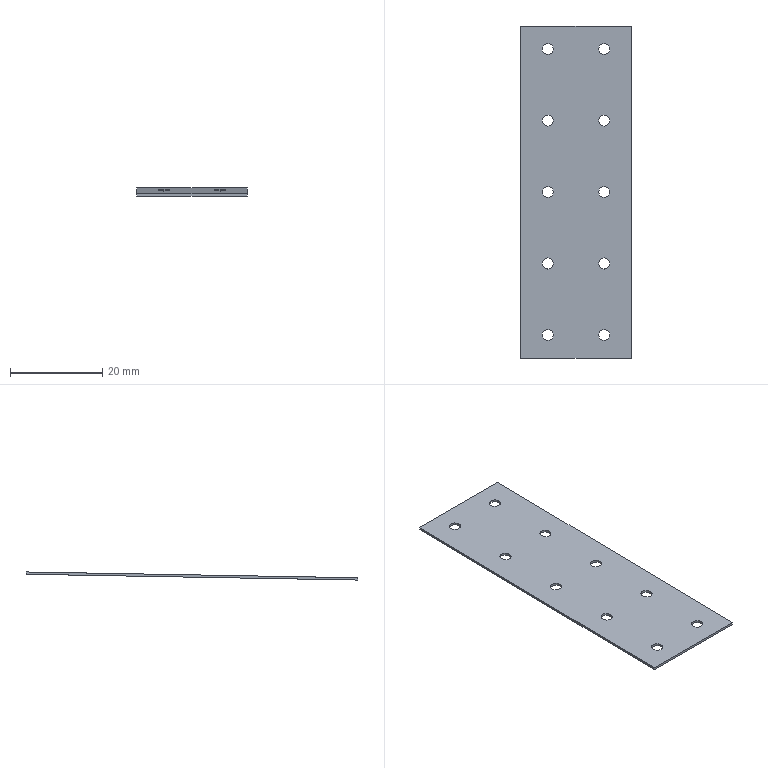Part | SolidWorks | features BaseBody 1 | 1 solid | 26 faces | box 24 x 71.993 x 1.756 mm | volume 841.326 mm3 | cylinder 20 | plane 6 | commonest cylinder face diameters 2.4 x20
STEP:
#1=CARTESIAN_POINT('',(-1405.625,-3.837,-0.5671));
#2=VERTEX_POINT('',#1);
#3=CARTESIAN_POINT('',(-1405.625,-1.437,-0.5252));
#4=VERTEX_POINT('',#3);
#5=CARTESIAN_POINT('',(-1405.625,-2.637,-0.5461));
#6=DIRECTION('',(0.,0.01745,-0.9998));
#7=DIRECTION('',(0.,-0.9998,-0.01745));
#8=AXIS2_PLACEMENT_3D('',#5,#6,#7);
#9=CIRCLE('',#8,1.2);
#10=EDGE_CURVE('',#2,#4,#9,.T.);
#11=ORIENTED_EDGE('',*,*,#10,.T.);
#12=CARTESIAN_POINT('',(-1405.625,-1.446,-0.02524));
#13=VERTEX_POINT('',#12);
#14=CARTESIAN_POINT('',(-1405.625,-1.437,-0.5252));
#15=DIRECTION('',(0.,-0.01745,0.9998));
#16=VECTOR('',#15,1000.);
#17=LINE('',#14,#16);
#18=EDGE_CURVE('',#4,#13,#17,.T.);
#19=ORIENTED_EDGE('',*,*,#18,.T.);
#20=CARTESIAN_POINT('',(-1405.625,-3.846,-0.06713));
#21=VERTEX_POINT('',#20);
#22=CARTESIAN_POINT('',(-1405.625,-2.646,-0.04619));
#23=DIRECTION('',(0.,-0.01745,0.9998));
#24=DIRECTION('',(0.,-0.9998,-0.01745));
#25=AXIS2_PLACEMENT_3D('',#22,#23,#24);
#26=CIRCLE('',#25,1.2);
#27=EDGE_CURVE('',#13,#21,#26,.T.);
#28=ORIENTED_EDGE('',*,*,#27,.T.);
#29=CARTESIAN_POINT('',(-1405.625,-3.837,-0.5671));
#30=DIRECTION('',(0.,-0.01745,0.9998));
#31=VECTOR('',#30,1000.);
#32=LINE('',#29,#31);
#33=EDGE_CURVE('',#2,#21,#32,.T.);
#34=ORIENTED_EDGE('',*,*,#33,.F.);
#35=EDGE_LOOP('',(#11,#19,#28,#34));
#36=FACE_OUTER_BOUND('',#35,.T.);
#37=CARTESIAN_POINT('',(-1405.625,-2.637,-0.5461));
#38=DIRECTION('',(0.,-0.01745,0.9998));
#39=DIRECTION('',(0.,-0.9998,-0.01745));
#40=AXIS2_PLACEMENT_3D('',#37,#38,#39);
#41=CYLINDRICAL_SURFACE('',#40,1.2);
#42=ADVANCED_FACE('',(#36),#41,.F.);
#43=CARTESIAN_POINT('',(-1417.875,27.156,-0.02607));
#44=VERTEX_POINT('',#43);
#45=CARTESIAN_POINT('',(-1417.875,29.556,0.01582));
#46=VERTEX_POINT('',#45);
#47=CARTESIAN_POINT('',(-1417.875,28.356,-0.005126));
#48=DIRECTION('',(0.,0.01745,-0.9998));
#49=DIRECTION('',(0.,-0.9998,-0.01745));
#50=AXIS2_PLACEMENT_3D('',#47,#48,#49);
#51=CIRCLE('',#50,1.2);
#52=EDGE_CURVE('',#44,#46,#51,.T.);
#53=ORIENTED_EDGE('',*,*,#52,.T.);
#54=CARTESIAN_POINT('',(-1417.875,29.547,0.5157));
#55=VERTEX_POINT('',#54);
#56=CARTESIAN_POINT('',(-1417.875,29.556,0.01582));
#57=DIRECTION('',(0.,-0.01745,0.9998));
#58=VECTOR('',#57,1000.);
#59=LINE('',#56,#58);
#60=EDGE_CURVE('',#46,#55,#59,.T.);
#61=ORIENTED_EDGE('',*,*,#60,.T.);
#62=CARTESIAN_POINT('',(-1417.875,27.147,0.4739));
#63=VERTEX_POINT('',#62);
#64=CARTESIAN_POINT('',(-1417.875,28.347,0.4948));
#65=DIRECTION('',(0.,0.01745,-0.9998));
#66=DIRECTION('',(0.,-0.9998,-0.01745));
#67=AXIS2_PLACEMENT_3D('',#64,#65,#66);
#68=CIRCLE('',#67,1.2);
#69=EDGE_CURVE('',#63,#55,#68,.T.);
#70=ORIENTED_EDGE('',*,*,#69,.F.);
#71=CARTESIAN_POINT('',(-1417.875,27.156,-0.02607));
#72=DIRECTION('',(0.,-0.01745,0.9998));
#73=VECTOR('',#72,1000.);
#74=LINE('',#71,#73);
#75=EDGE_CURVE('',#44,#63,#74,.T.);
#76=ORIENTED_EDGE('',*,*,#75,.F.);
#77=EDGE_LOOP('',(#53,#61,#70,#76));
#78=FACE_OUTER_BOUND('',#77,.T.);
#79=CARTESIAN_POINT('',(-1417.875,28.356,-0.005126));
#80=DIRECTION('',(0.,-0.01745,0.9998));
#81=DIRECTION('',(0.,-0.9998,-0.01745));
#82=AXIS2_PLACEMENT_3D('',#79,#80,#81);
#83=CYLINDRICAL_SURFACE('',#82,1.2);
#84=ADVANCED_FACE('',(#78),#83,.F.);
#85=CARTESIAN_POINT('',(-1417.875,11.659,-0.2966));
#86=VERTEX_POINT('',#85);
#87=CARTESIAN_POINT('',(-1417.875,14.059,-0.2547));
#88=VERTEX_POINT('',#87);
#89=CARTESIAN_POINT('',(-1417.875,12.859,-0.2756));
#90=DIRECTION('',(0.,0.01745,-0.9998));
#91=DIRECTION('',(0.,-0.9998,-0.01745));
#92=AXIS2_PLACEMENT_3D('',#89,#90,#91);
#93=CIRCLE('',#92,1.2);
#94=EDGE_CURVE('',#86,#88,#93,.T.);
#95=ORIENTED_EDGE('',*,*,#94,.T.);
#96=CARTESIAN_POINT('',(-1417.875,14.05,0.2452));
#97=VERTEX_POINT('',#96);
#98=CARTESIAN_POINT('',(-1417.875,14.059,-0.2547));
#99=DIRECTION('',(0.,-0.01745,0.9998));
#100=VECTOR('',#99,1000.);
#101=LINE('',#98,#100);
#102=EDGE_CURVE('',#88,#97,#101,.T.);
#103=ORIENTED_EDGE('',*,*,#102,.T.);
#104=CARTESIAN_POINT('',(-1417.875,11.651,0.2034));
#105=VERTEX_POINT('',#104);
#106=CARTESIAN_POINT('',(-1417.875,12.85,0.2243));
#107=DIRECTION('',(0.,0.01745,-0.9998));
#108=DIRECTION('',(0.,-0.9998,-0.01745));
#109=AXIS2_PLACEMENT_3D('',#106,#107,#108);
#110=CIRCLE('',#109,1.2);
#111=EDGE_CURVE('',#105,#97,#110,.T.);
#112=ORIENTED_EDGE('',*,*,#111,.F.);
#113=CARTESIAN_POINT('',(-1417.875,11.659,-0.2966));
#114=DIRECTION('',(0.,-0.01745,0.9998));
#115=VECTOR('',#114,1000.);
#116=LINE('',#113,#115);
#117=EDGE_CURVE('',#86,#105,#116,.T.);
#118=ORIENTED_EDGE('',*,*,#117,.F.);
#119=EDGE_LOOP('',(#95,#103,#112,#118));
#120=FACE_OUTER_BOUND('',#119,.T.);
#121=CARTESIAN_POINT('',(-1417.875,12.859,-0.2756));
#122=DIRECTION('',(0.,-0.01745,0.9998));
#123=DIRECTION('',(0.,-0.9998,-0.01745));
#124=AXIS2_PLACEMENT_3D('',#121,#122,#123);
#125=CYLINDRICAL_SURFACE('',#124,1.2);
#126=ADVANCED_FACE('',(#120),#125,.F.);
#127=CARTESIAN_POINT('',(-1405.625,-19.334,-0.8375));
#128=VERTEX_POINT('',#127);
#129=CARTESIAN_POINT('',(-1405.625,-16.934,-0.7957));
#130=VERTEX_POINT('',#129);
#131=CARTESIAN_POINT('',(-1405.625,-18.134,-0.8166));
#132=DIRECTION('',(0.,0.01745,-0.9998));
#133=DIRECTION('',(0.,-0.9998,-0.01745));
#134=AXIS2_PLACEMENT_3D('',#131,#132,#133);
#135=CIRCLE('',#134,1.2);
#136=EDGE_CURVE('',#128,#130,#135,.T.);
#137=ORIENTED_EDGE('',*,*,#136,.T.);
#138=CARTESIAN_POINT('',(-1405.625,-16.943,-0.2957));
#139=VERTEX_POINT('',#138);
#140=CARTESIAN_POINT('',(-1405.625,-16.934,-0.7957));
#141=DIRECTION('',(0.,-0.01745,0.9998));
#142=VECTOR('',#141,1000.);
#143=LINE('',#140,#142);
#144=EDGE_CURVE('',#130,#139,#143,.T.);
#145=ORIENTED_EDGE('',*,*,#144,.T.);
#146=CARTESIAN_POINT('',(-1405.625,-19.342,-0.3376));
#147=VERTEX_POINT('',#146);
#148=CARTESIAN_POINT('',(-1405.625,-18.143,-0.3167));
#149=DIRECTION('',(0.,0.01745,-0.9998));
#150=DIRECTION('',(0.,-0.9998,-0.01745));
#151=AXIS2_PLACEMENT_3D('',#148,#149,#150);
#152=CIRCLE('',#151,1.2);
#153=EDGE_CURVE('',#147,#139,#152,.T.);
#154=ORIENTED_EDGE('',*,*,#153,.F.);
#155=CARTESIAN_POINT('',(-1405.625,-19.334,-0.8375));
#156=DIRECTION('',(0.,-0.01745,0.9998));
#157=VECTOR('',#156,1000.);
#158=LINE('',#155,#157);
#159=EDGE_CURVE('',#128,#147,#158,.T.);
#160=ORIENTED_EDGE('',*,*,#159,.F.);
#161=EDGE_LOOP('',(#137,#145,#154,#160));
#162=FACE_OUTER_BOUND('',#161,.T.);
#163=CARTESIAN_POINT('',(-1405.625,-18.134,-0.8166));
#164=DIRECTION('',(0.,-0.01745,0.9998));
#165=DIRECTION('',(0.,-0.9998,-0.01745));
#166=AXIS2_PLACEMENT_3D('',#163,#164,#165);
#167=CYLINDRICAL_SURFACE('',#166,1.2);
#168=ADVANCED_FACE('',(#162),#167,.F.);
#169=CARTESIAN_POINT('',(-1417.875,42.652,0.2444));
#170=VERTEX_POINT('',#169);
#171=CARTESIAN_POINT('',(-1417.875,45.052,0.2863));
#172=VERTEX_POINT('',#171);
#173=CARTESIAN_POINT('',(-1417.875,43.852,0.2654));
#174=DIRECTION('',(0.,0.01745,-0.9998));
#175=DIRECTION('',(0.,-0.9998,-0.01745));
#176=AXIS2_PLACEMENT_3D('',#173,#174,#175);
#177=CIRCLE('',#176,1.2);
#178=EDGE_CURVE('',#170,#172,#177,.T.);
#179=ORIENTED_EDGE('',*,*,#178,.T.);
#180=CARTESIAN_POINT('',(-1417.875,45.043,0.7862));
#181=VERTEX_POINT('',#180);
#182=CARTESIAN_POINT('',(-1417.875,45.052,0.2863));
#183=DIRECTION('',(0.,-0.01745,0.9998));
#184=VECTOR('',#183,1000.);
#185=LINE('',#182,#184);
#186=EDGE_CURVE('',#172,#181,#185,.T.);
#187=ORIENTED_EDGE('',*,*,#186,.T.);
#188=CARTESIAN_POINT('',(-1417.875,42.644,0.7443));
#189=VERTEX_POINT('',#188);
#190=CARTESIAN_POINT('',(-1417.875,43.843,0.7653));
#191=DIRECTION('',(0.,0.01745,-0.9998));
#192=DIRECTION('',(0.,-0.9998,-0.01745));
#193=AXIS2_PLACEMENT_3D('',#190,#191,#192);
#194=CIRCLE('',#193,1.2);
#195=EDGE_CURVE('',#189,#181,#194,.T.);
#196=ORIENTED_EDGE('',*,*,#195,.F.);
#197=CARTESIAN_POINT('',(-1417.875,42.652,0.2444));
#198=DIRECTION('',(0.,-0.01745,0.9998));
#199=VECTOR('',#198,1000.);
#200=LINE('',#197,#199);
#201=EDGE_CURVE('',#170,#189,#200,.T.);
#202=ORIENTED_EDGE('',*,*,#201,.F.);
#203=EDGE_LOOP('',(#179,#187,#196,#202));
#204=FACE_OUTER_BOUND('',#203,.T.);
#205=CARTESIAN_POINT('',(-1417.875,43.852,0.2654));
#206=DIRECTION('',(0.,-0.01745,0.9998));
#207=DIRECTION('',(0.,-0.9998,-0.01745));
#208=AXIS2_PLACEMENT_3D('',#205,#206,#207);
#209=CYLINDRICAL_SURFACE('',#208,1.2);
#210=ADVANCED_FACE('',(#204),#209,.F.);
#211=CARTESIAN_POINT('',(-1405.625,42.652,0.2444));
#212=VERTEX_POINT('',#211);
#213=CARTESIAN_POINT('',(-1405.625,45.052,0.2863));
#214=VERTEX_POINT('',#213);
#215=CARTESIAN_POINT('',(-1405.625,43.852,0.2654));
#216=DIRECTION('',(0.,0.01745,-0.9998));
#217=DIRECTION('',(0.,-0.9998,-0.01745));
#218=AXIS2_PLACEMENT_3D('',#215,#216,#217);
#219=CIRCLE('',#218,1.2);
#220=EDGE_CURVE('',#212,#214,#219,.T.);
#221=ORIENTED_EDGE('',*,*,#220,.T.);
#222=CARTESIAN_POINT('',(-1405.625,45.043,0.7862));
#223=VERTEX_POINT('',#222);
#224=CARTESIAN_POINT('',(-1405.625,45.052,0.2863));
#225=DIRECTION('',(0.,-0.01745,0.9998));
#226=VECTOR('',#225,1000.);
#227=LINE('',#224,#226);
#228=EDGE_CURVE('',#214,#223,#227,.T.);
#229=ORIENTED_EDGE('',*,*,#228,.T.);
#230=CARTESIAN_POINT('',(-1405.625,42.644,0.7443));
#231=VERTEX_POINT('',#230);
#232=CARTESIAN_POINT('',(-1405.625,43.843,0.7653));
#233=DIRECTION('',(0.,0.01745,-0.9998));
#234=DIRECTION('',(0.,-0.9998,-0.01745));
#235=AXIS2_PLACEMENT_3D('',#232,#233,#234);
#236=CIRCLE('',#235,1.2);
#237=EDGE_CURVE('',#231,#223,#236,.T.);
#238=ORIENTED_EDGE('',*,*,#237,.F.);
#239=CARTESIAN_POINT('',(-1405.625,42.652,0.2444));
#240=DIRECTION('',(0.,-0.01745,0.9998));
#241=VECTOR('',#240,1000.);
#242=LINE('',#239,#241);
#243=EDGE_CURVE('',#212,#231,#242,.T.);
#244=ORIENTED_EDGE('',*,*,#243,.F.);
#245=EDGE_LOOP('',(#221,#229,#238,#244));
#246=FACE_OUTER_BOUND('',#245,.T.);
#247=CARTESIAN_POINT('',(-1405.625,43.852,0.2654));
#248=DIRECTION('',(0.,-0.01745,0.9998));
#249=DIRECTION('',(0.,-0.9998,-0.01745));
#250=AXIS2_PLACEMENT_3D('',#247,#248,#249);
#251=CYLINDRICAL_SURFACE('',#250,1.2);
#252=ADVANCED_FACE('',(#246),#251,.F.);
#253=CARTESIAN_POINT('',(-1417.875,-19.334,-0.8375));
#254=VERTEX_POINT('',#253);
#255=CARTESIAN_POINT('',(-1417.875,-16.934,-0.7957));
#256=VERTEX_POINT('',#255);
#257=CARTESIAN_POINT('',(-1417.875,-18.134,-0.8166));
#258=DIRECTION('',(0.,0.01745,-0.9998));
#259=DIRECTION('',(0.,-0.9998,-0.01745));
#260=AXIS2_PLACEMENT_3D('',#257,#258,#259);
#261=CIRCLE('',#260,1.2);
#262=EDGE_CURVE('',#254,#256,#261,.T.);
#263=ORIENTED_EDGE('',*,*,#262,.T.);
#264=CARTESIAN_POINT('',(-1417.875,-16.943,-0.2957));
#265=VERTEX_POINT('',#264);
#266=CARTESIAN_POINT('',(-1417.875,-16.934,-0.7957));
#267=DIRECTION('',(0.,-0.01745,0.9998));
#268=VECTOR('',#267,1000.);
#269=LINE('',#266,#268);
#270=EDGE_CURVE('',#256,#265,#269,.T.);
#271=ORIENTED_EDGE('',*,*,#270,.T.);
#272=CARTESIAN_POINT('',(-1417.875,-19.342,-0.3376));
#273=VERTEX_POINT('',#272);
#274=CARTESIAN_POINT('',(-1417.875,-18.143,-0.3167));
#275=DIRECTION('',(0.,0.01745,-0.9998));
#276=DIRECTION('',(0.,-0.9998,-0.01745));
#277=AXIS2_PLACEMENT_3D('',#274,#275,#276);
#278=CIRCLE('',#277,1.2);
#279=EDGE_CURVE('',#273,#265,#278,.T.);
#280=ORIENTED_EDGE('',*,*,#279,.F.);
#281=CARTESIAN_POINT('',(-1417.875,-19.334,-0.8375));
#282=DIRECTION('',(0.,-0.01745,0.9998));
#283=VECTOR('',#282,1000.);
#284=LINE('',#281,#283);
#285=EDGE_CURVE('',#254,#273,#284,.T.);
#286=ORIENTED_EDGE('',*,*,#285,.F.);
#287=EDGE_LOOP('',(#263,#271,#280,#286));
#288=FACE_OUTER_BOUND('',#287,.T.);
#289=CARTESIAN_POINT('',(-1417.875,-18.134,-0.8166));
#290=DIRECTION('',(0.,-0.01745,0.9998));
#291=DIRECTION('',(0.,-0.9998,-0.01745));
#292=AXIS2_PLACEMENT_3D('',#289,#290,#291);
#293=CYLINDRICAL_SURFACE('',#292,1.2);
#294=ADVANCED_FACE('',(#288),#293,.F.);
#295=CARTESIAN_POINT('',(-1405.625,11.659,-0.2966));
#296=VERTEX_POINT('',#295);
#297=CARTESIAN_POINT('',(-1405.625,14.059,-0.2547));
#298=VERTEX_POINT('',#297);
#299=CARTESIAN_POINT('',(-1405.625,12.859,-0.2756));
#300=DIRECTION('',(0.,0.01745,-0.9998));
#301=DIRECTION('',(0.,-0.9998,-0.01745));
#302=AXIS2_PLACEMENT_3D('',#299,#300,#301);
#303=CIRCLE('',#302,1.2);
#304=EDGE_CURVE('',#296,#298,#303,.T.);
#305=ORIENTED_EDGE('',*,*,#304,.T.);
#306=CARTESIAN_POINT('',(-1405.625,14.05,0.2452));
#307=VERTEX_POINT('',#306);
#308=CARTESIAN_POINT('',(-1405.625,14.059,-0.2547));
#309=DIRECTION('',(0.,-0.01745,0.9998));
#310=VECTOR('',#309,1000.);
#311=LINE('',#308,#310);
#312=EDGE_CURVE('',#298,#307,#311,.T.);
#313=ORIENTED_EDGE('',*,*,#312,.T.);
#314=CARTESIAN_POINT('',(-1405.625,11.651,0.2034));
#315=VERTEX_POINT('',#314);
#316=CARTESIAN_POINT('',(-1405.625,12.85,0.2243));
#317=DIRECTION('',(0.,0.01745,-0.9998));
#318=DIRECTION('',(0.,-0.9998,-0.01745));
#319=AXIS2_PLACEMENT_3D('',#316,#317,#318);
#320=CIRCLE('',#319,1.2);
#321=EDGE_CURVE('',#315,#307,#320,.T.);
#322=ORIENTED_EDGE('',*,*,#321,.F.);
#323=CARTESIAN_POINT('',(-1405.625,11.659,-0.2966));
#324=DIRECTION('',(0.,-0.01745,0.9998));
#325=VECTOR('',#324,1000.);
#326=LINE('',#323,#325);
#327=EDGE_CURVE('',#296,#315,#326,.T.);
#328=ORIENTED_EDGE('',*,*,#327,.F.);
#329=EDGE_LOOP('',(#305,#313,#322,#328));
#330=FACE_OUTER_BOUND('',#329,.T.);
#331=CARTESIAN_POINT('',(-1405.625,12.859,-0.2756));
#332=DIRECTION('',(0.,-0.01745,0.9998));
#333=DIRECTION('',(0.,-0.9998,-0.01745));
#334=AXIS2_PLACEMENT_3D('',#331,#332,#333);
#335=CYLINDRICAL_SURFACE('',#334,1.2);
#336=ADVANCED_FACE('',(#330),#335,.F.);
#337=CARTESIAN_POINT('',(-1405.625,27.156,-0.02607));
#338=VERTEX_POINT('',#337);
#339=CARTESIAN_POINT('',(-1405.625,29.556,0.01582));
#340=VERTEX_POINT('',#339);
#341=CARTESIAN_POINT('',(-1405.625,28.356,-0.005126));
#342=DIRECTION('',(0.,0.01745,-0.9998));
#343=DIRECTION('',(0.,-0.9998,-0.01745));
#344=AXIS2_PLACEMENT_3D('',#341,#342,#343);
#345=CIRCLE('',#344,1.2);
#346=EDGE_CURVE('',#338,#340,#345,.T.);
#347=ORIENTED_EDGE('',*,*,#346,.T.);
#348=CARTESIAN_POINT('',(-1405.625,29.547,0.5157));
#349=VERTEX_POINT('',#348);
#350=CARTESIAN_POINT('',(-1405.625,29.556,0.01582));
#351=DIRECTION('',(0.,-0.01745,0.9998));
#352=VECTOR('',#351,1000.);
#353=LINE('',#350,#352);
#354=EDGE_CURVE('',#340,#349,#353,.T.);
#355=ORIENTED_EDGE('',*,*,#354,.T.);
#356=CARTESIAN_POINT('',(-1405.625,27.147,0.4739));
#357=VERTEX_POINT('',#356);
#358=CARTESIAN_POINT('',(-1405.625,28.347,0.4948));
#359=DIRECTION('',(0.,0.01745,-0.9998));
#360=DIRECTION('',(0.,-0.9998,-0.01745));
#361=AXIS2_PLACEMENT_3D('',#358,#359,#360);
#362=CIRCLE('',#361,1.2);
#363=EDGE_CURVE('',#357,#349,#362,.T.);
#364=ORIENTED_EDGE('',*,*,#363,.F.);
#365=CARTESIAN_POINT('',(-1405.625,27.156,-0.02607));
#366=DIRECTION('',(0.,-0.01745,0.9998));
#367=VECTOR('',#366,1000.);
#368=LINE('',#365,#367);
#369=EDGE_CURVE('',#338,#357,#368,.T.);
#370=ORIENTED_EDGE('',*,*,#369,.F.);
#371=EDGE_LOOP('',(#347,#355,#364,#370));
#372=FACE_OUTER_BOUND('',#371,.T.);
#373=CARTESIAN_POINT('',(-1405.625,28.356,-0.005126));
#374=DIRECTION('',(0.,-0.01745,0.9998));
#375=DIRECTION('',(0.,-0.9998,-0.01745));
#376=AXIS2_PLACEMENT_3D('',#373,#374,#375);
#377=CYLINDRICAL_SURFACE('',#376,1.2);
#378=ADVANCED_FACE('',(#372),#377,.F.);
#379=CARTESIAN_POINT('',(-1417.875,-3.837,-0.5671));
#380=VERTEX_POINT('',#379);
#381=CARTESIAN_POINT('',(-1417.875,-1.437,-0.5252));
#382=VERTEX_POINT('',#381);
#383=CARTESIAN_POINT('',(-1417.875,-2.637,-0.5461));
#384=DIRECTION('',(0.,0.01745,-0.9998));
#385=DIRECTION('',(0.,-0.9998,-0.01745));
#386=AXIS2_PLACEMENT_3D('',#383,#384,#385);
#387=CIRCLE('',#386,1.2);
#388=EDGE_CURVE('',#380,#382,#387,.T.);
#389=ORIENTED_EDGE('',*,*,#388,.T.);
#390=CARTESIAN_POINT('',(-1417.875,-1.446,-0.02524));
#391=VERTEX_POINT('',#390);
#392=CARTESIAN_POINT('',(-1417.875,-1.437,-0.5252));
#393=DIRECTION('',(0.,-0.01745,0.9998));
#394=VECTOR('',#393,1000.);
#395=LINE('',#392,#394);
#396=EDGE_CURVE('',#382,#391,#395,.T.);
#397=ORIENTED_EDGE('',*,*,#396,.T.);
#398=CARTESIAN_POINT('',(-1417.875,-3.846,-0.06713));
#399=VERTEX_POINT('',#398);
#400=CARTESIAN_POINT('',(-1417.875,-2.646,-0.04619));
#401=DIRECTION('',(0.,0.01745,-0.9998));
#402=DIRECTION('',(0.,-0.9998,-0.01745));
#403=AXIS2_PLACEMENT_3D('',#400,#401,#402);
#404=CIRCLE('',#403,1.2);
#405=EDGE_CURVE('',#399,#391,#404,.T.);
#406=ORIENTED_EDGE('',*,*,#405,.F.);
#407=CARTESIAN_POINT('',(-1417.875,-3.837,-0.5671));
#408=DIRECTION('',(0.,-0.01745,0.9998));
#409=VECTOR('',#408,1000.);
#410=LINE('',#407,#409);
#411=EDGE_CURVE('',#380,#399,#410,.T.);
#412=ORIENTED_EDGE('',*,*,#411,.F.);
#413=EDGE_LOOP('',(#389,#397,#406,#412));
#414=FACE_OUTER_BOUND('',#413,.T.);
#415=CARTESIAN_POINT('',(-1417.875,-2.637,-0.5461));
#416=DIRECTION('',(0.,-0.01745,0.9998));
#417=DIRECTION('',(0.,-0.9998,-0.01745));
#418=AXIS2_PLACEMENT_3D('',#415,#416,#417);
#419=CYLINDRICAL_SURFACE('',#418,1.2);
#420=ADVANCED_FACE('',(#414),#419,.F.);
#421=ORIENTED_EDGE('',*,*,#18,.F.);
#422=CARTESIAN_POINT('',(-1405.625,-2.637,-0.5461));
#423=DIRECTION('',(0.,0.01745,-0.9998));
#424=DIRECTION('',(0.,-0.9998,-0.01745));
#425=AXIS2_PLACEMENT_3D('',#422,#423,#424);
#426=CIRCLE('',#425,1.2);
#427=EDGE_CURVE('',#4,#2,#426,.T.);
#428=ORIENTED_EDGE('',*,*,#427,.T.);
#429=ORIENTED_EDGE('',*,*,#33,.T.);
#430=CARTESIAN_POINT('',(-1405.625,-2.646,-0.04619));
#431=DIRECTION('',(0.,-0.01745,0.9998));
#432=DIRECTION('',(0.,-0.9998,-0.01745));
#433=AXIS2_PLACEMENT_3D('',#430,#431,#432);
#434=CIRCLE('',#433,1.2);
#435=EDGE_CURVE('',#21,#13,#434,.T.);
#436=ORIENTED_EDGE('',*,*,#435,.T.);
#437=EDGE_LOOP('',(#421,#428,#429,#436));
#438=FACE_OUTER_BOUND('',#437,.T.);
#439=CARTESIAN_POINT('',(-1405.625,-2.637,-0.5461));
#440=DIRECTION('',(0.,-0.01745,0.9998));
#441=DIRECTION('',(0.,-0.9998,-0.01745));
#442=AXIS2_PLACEMENT_3D('',#439,#440,#441);
#443=CYLINDRICAL_SURFACE('',#442,1.2);
#444=ADVANCED_FACE('',(#438),#443,.F.);
#445=ORIENTED_EDGE('',*,*,#435,.F.);
#446=ORIENTED_EDGE('',*,*,#27,.F.);
#447=EDGE_LOOP('',(#445,#446));
#448=FACE_BOUND('',#447,.T.);
#449=ORIENTED_EDGE('',*,*,#69,.T.);
#450=CARTESIAN_POINT('',(-1417.875,28.347,0.4948));
#451=DIRECTION('',(0.,0.01745,-0.9998));
#452=DIRECTION('',(0.,-0.9998,-0.01745));
#453=AXIS2_PLACEMENT_3D('',#450,#451,#452);
#454=CIRCLE('',#453,1.2);
#455=EDGE_CURVE('',#55,#63,#454,.T.);
#456=ORIENTED_EDGE('',*,*,#455,.T.);
#457=EDGE_LOOP('',(#449,#456));
#458=FACE_BOUND('',#457,.T.);
#459=ORIENTED_EDGE('',*,*,#111,.T.);
#460=CARTESIAN_POINT('',(-1417.875,12.85,0.2243));
#461=DIRECTION('',(0.,0.01745,-0.9998));
#462=DIRECTION('',(0.,-0.9998,-0.01745));
#463=AXIS2_PLACEMENT_3D('',#460,#461,#462);
#464=CIRCLE('',#463,1.2);
#465=EDGE_CURVE('',#97,#105,#464,.T.);
#466=ORIENTED_EDGE('',*,*,#465,.T.);
#467=EDGE_LOOP('',(#459,#466));
#468=FACE_BOUND('',#467,.T.);
#469=ORIENTED_EDGE('',*,*,#153,.T.);
#470=CARTESIAN_POINT('',(-1405.625,-18.143,-0.3167));
#471=DIRECTION('',(0.,0.01745,-0.9998));
#472=DIRECTION('',(0.,-0.9998,-0.01745));
#473=AXIS2_PLACEMENT_3D('',#470,#471,#472);
#474=CIRCLE('',#473,1.2);
#475=EDGE_CURVE('',#139,#147,#474,.T.);
#476=ORIENTED_EDGE('',*,*,#475,.T.);
#477=EDGE_LOOP('',(#469,#476));
#478=FACE_BOUND('',#477,.T.);
#479=ORIENTED_EDGE('',*,*,#195,.T.);
#480=CARTESIAN_POINT('',(-1417.875,43.843,0.7653));
#481=DIRECTION('',(0.,0.01745,-0.9998));
#482=DIRECTION('',(0.,-0.9998,-0.01745));
#483=AXIS2_PLACEMENT_3D('',#480,#481,#482);
#484=CIRCLE('',#483,1.2);
#485=EDGE_CURVE('',#181,#189,#484,.T.);
#486=ORIENTED_EDGE('',*,*,#485,.T.);
#487=EDGE_LOOP('',(#479,#486));
#488=FACE_BOUND('',#487,.T.);
#489=ORIENTED_EDGE('',*,*,#237,.T.);
#490=CARTESIAN_POINT('',(-1405.625,43.843,0.7653));
#491=DIRECTION('',(0.,0.01745,-0.9998));
#492=DIRECTION('',(0.,-0.9998,-0.01745));
#493=AXIS2_PLACEMENT_3D('',#490,#491,#492);
#494=CIRCLE('',#493,1.2);
#495=EDGE_CURVE('',#223,#231,#494,.T.);
#496=ORIENTED_EDGE('',*,*,#495,.T.);
#497=EDGE_LOOP('',(#489,#496));
#498=FACE_BOUND('',#497,.T.);
#499=ORIENTED_EDGE('',*,*,#279,.T.);
#500=CARTESIAN_POINT('',(-1417.875,-18.143,-0.3167));
#501=DIRECTION('',(0.,0.01745,-0.9998));
#502=DIRECTION('',(0.,-0.9998,-0.01745));
#503=AXIS2_PLACEMENT_3D('',#500,#501,#502);
#504=CIRCLE('',#503,1.2);
#505=EDGE_CURVE('',#265,#273,#504,.T.);
#506=ORIENTED_EDGE('',*,*,#505,.T.);
#507=EDGE_LOOP('',(#499,#506));
#508=FACE_BOUND('',#507,.T.);
#509=ORIENTED_EDGE('',*,*,#321,.T.);
#510=CARTESIAN_POINT('',(-1405.625,12.85,0.2243));
#511=DIRECTION('',(0.,0.01745,-0.9998));
#512=DIRECTION('',(0.,-0.9998,-0.01745));
#513=AXIS2_PLACEMENT_3D('',#510,#511,#512);
#514=CIRCLE('',#513,1.2);
#515=EDGE_CURVE('',#307,#315,#514,.T.);
#516=ORIENTED_EDGE('',*,*,#515,.T.);
#517=EDGE_LOOP('',(#509,#516));
#518=FACE_BOUND('',#517,.T.);
#519=ORIENTED_EDGE('',*,*,#363,.T.);
#520=CARTESIAN_POINT('',(-1405.625,28.347,0.4948));
#521=DIRECTION('',(0.,0.01745,-0.9998));
#522=DIRECTION('',(0.,-0.9998,-0.01745));
#523=AXIS2_PLACEMENT_3D('',#520,#521,#522);
#524=CIRCLE('',#523,1.2);
#525=EDGE_CURVE('',#349,#357,#524,.T.);
#526=ORIENTED_EDGE('',*,*,#525,.T.);
#527=EDGE_LOOP('',(#519,#526));
#528=FACE_BOUND('',#527,.T.);
#529=ORIENTED_EDGE('',*,*,#405,.T.);
#530=CARTESIAN_POINT('',(-1417.875,-2.646,-0.04619));
#531=DIRECTION('',(0.,0.01745,-0.9998));
#532=DIRECTION('',(0.,-0.9998,-0.01745));
#533=AXIS2_PLACEMENT_3D('',#530,#531,#532);
#534=CIRCLE('',#533,1.2);
#535=EDGE_CURVE('',#391,#399,#534,.T.);
#536=ORIENTED_EDGE('',*,*,#535,.T.);
#537=EDGE_LOOP('',(#529,#536));
#538=FACE_BOUND('',#537,.T.);
#539=CARTESIAN_POINT('',(-1423.75,48.843,0.8526));
#540=VERTEX_POINT('',#539);
#541=CARTESIAN_POINT('',(-1423.75,-23.142,-0.4039));
#542=VERTEX_POINT('',#541);
#543=CARTESIAN_POINT('',(-1423.75,12.85,0.2243));
#544=DIRECTION('',(0.,-0.9998,-0.01745));
#545=VECTOR('',#544,1000.);
#546=LINE('',#543,#545);
#547=EDGE_CURVE('',#540,#542,#546,.T.);
#548=ORIENTED_EDGE('',*,*,#547,.T.);
#549=CARTESIAN_POINT('',(-1399.75,-23.142,-0.4039));
#550=VERTEX_POINT('',#549);
#551=CARTESIAN_POINT('',(-1411.75,-23.142,-0.4039));
#552=DIRECTION('',(1.,0.,0.));
#553=VECTOR('',#552,1000.);
#554=LINE('',#551,#553);
#555=EDGE_CURVE('',#542,#550,#554,.T.);
#556=ORIENTED_EDGE('',*,*,#555,.T.);
#557=CARTESIAN_POINT('',(-1399.75,48.843,0.8526));
#558=VERTEX_POINT('',#557);
#559=CARTESIAN_POINT('',(-1399.75,12.85,0.2243));
#560=DIRECTION('',(0.,0.9998,0.01745));
#561=VECTOR('',#560,1000.);
#562=LINE('',#559,#561);
#563=EDGE_CURVE('',#550,#558,#562,.T.);
#564=ORIENTED_EDGE('',*,*,#563,.T.);
#565=CARTESIAN_POINT('',(-1411.75,48.843,0.8526));
#566=DIRECTION('',(-1.,0.,0.));
#567=VECTOR('',#566,1000.);
#568=LINE('',#565,#567);
#569=EDGE_CURVE('',#558,#540,#568,.T.);
#570=ORIENTED_EDGE('',*,*,#569,.T.);
#571=EDGE_LOOP('',(#548,#556,#564,#570));
#572=FACE_OUTER_BOUND('',#571,.T.);
#573=CARTESIAN_POINT('',(-1423.75,48.843,0.8526));
#574=DIRECTION('',(0.,-0.01745,0.9998));
#575=DIRECTION('',(0.,-0.9998,-0.01745));
#576=AXIS2_PLACEMENT_3D('',#573,#574,#575);
#577=PLANE('',#576);
#578=ADVANCED_FACE('',(#448,#458,#468,#478,#488,#498,#508,#518,#528,#538,#572),#577,.T.);
#579=ORIENTED_EDGE('',*,*,#10,.F.);
#580=ORIENTED_EDGE('',*,*,#427,.F.);
#581=EDGE_LOOP('',(#579,#580));
#582=FACE_BOUND('',#581,.T.);
#583=ORIENTED_EDGE('',*,*,#52,.F.);
#584=CARTESIAN_POINT('',(-1417.875,28.356,-0.005126));
#585=DIRECTION('',(0.,0.01745,-0.9998));
#586=DIRECTION('',(0.,-0.9998,-0.01745));
#587=AXIS2_PLACEMENT_3D('',#584,#585,#586);
#588=CIRCLE('',#587,1.2);
#589=EDGE_CURVE('',#46,#44,#588,.T.);
#590=ORIENTED_EDGE('',*,*,#589,.F.);
#591=EDGE_LOOP('',(#583,#590));
#592=FACE_BOUND('',#591,.T.);
#593=ORIENTED_EDGE('',*,*,#94,.F.);
#594=CARTESIAN_POINT('',(-1417.875,12.859,-0.2756));
#595=DIRECTION('',(0.,0.01745,-0.9998));
#596=DIRECTION('',(0.,-0.9998,-0.01745));
#597=AXIS2_PLACEMENT_3D('',#594,#595,#596);
#598=CIRCLE('',#597,1.2);
#599=EDGE_CURVE('',#88,#86,#598,.T.);
#600=ORIENTED_EDGE('',*,*,#599,.F.);
#601=EDGE_LOOP('',(#593,#600));
#602=FACE_BOUND('',#601,.T.);
#603=ORIENTED_EDGE('',*,*,#136,.F.);
#604=CARTESIAN_POINT('',(-1405.625,-18.134,-0.8166));
#605=DIRECTION('',(0.,0.01745,-0.9998));
#606=DIRECTION('',(0.,-0.9998,-0.01745));
#607=AXIS2_PLACEMENT_3D('',#604,#605,#606);
#608=CIRCLE('',#607,1.2);
#609=EDGE_CURVE('',#130,#128,#608,.T.);
#610=ORIENTED_EDGE('',*,*,#609,.F.);
#611=EDGE_LOOP('',(#603,#610));
#612=FACE_BOUND('',#611,.T.);
#613=ORIENTED_EDGE('',*,*,#178,.F.);
#614=CARTESIAN_POINT('',(-1417.875,43.852,0.2654));
#615=DIRECTION('',(0.,0.01745,-0.9998));
#616=DIRECTION('',(0.,-0.9998,-0.01745));
#617=AXIS2_PLACEMENT_3D('',#614,#615,#616);
#618=CIRCLE('',#617,1.2);
#619=EDGE_CURVE('',#172,#170,#618,.T.);
#620=ORIENTED_EDGE('',*,*,#619,.F.);
#621=EDGE_LOOP('',(#613,#620));
#622=FACE_BOUND('',#621,.T.);
#623=ORIENTED_EDGE('',*,*,#220,.F.);
#624=CARTESIAN_POINT('',(-1405.625,43.852,0.2654));
#625=DIRECTION('',(0.,0.01745,-0.9998));
#626=DIRECTION('',(0.,-0.9998,-0.01745));
#627=AXIS2_PLACEMENT_3D('',#624,#625,#626);
#628=CIRCLE('',#627,1.2);
#629=EDGE_CURVE('',#214,#212,#628,.T.);
#630=ORIENTED_EDGE('',*,*,#629,.F.);
#631=EDGE_LOOP('',(#623,#630));
#632=FACE_BOUND('',#631,.T.);
#633=ORIENTED_EDGE('',*,*,#262,.F.);
#634=CARTESIAN_POINT('',(-1417.875,-18.134,-0.8166));
#635=DIRECTION('',(0.,0.01745,-0.9998));
#636=DIRECTION('',(0.,-0.9998,-0.01745));
#637=AXIS2_PLACEMENT_3D('',#634,#635,#636);
#638=CIRCLE('',#637,1.2);
#639=EDGE_CURVE('',#256,#254,#638,.T.);
#640=ORIENTED_EDGE('',*,*,#639,.F.);
#641=EDGE_LOOP('',(#633,#640));
#642=FACE_BOUND('',#641,.T.);
#643=ORIENTED_EDGE('',*,*,#304,.F.);
#644=CARTESIAN_POINT('',(-1405.625,12.859,-0.2756));
#645=DIRECTION('',(0.,0.01745,-0.9998));
#646=DIRECTION('',(0.,-0.9998,-0.01745));
#647=AXIS2_PLACEMENT_3D('',#644,#645,#646);
#648=CIRCLE('',#647,1.2);
#649=EDGE_CURVE('',#298,#296,#648,.T.);
#650=ORIENTED_EDGE('',*,*,#649,.F.);
#651=EDGE_LOOP('',(#643,#650));
#652=FACE_BOUND('',#651,.T.);
#653=ORIENTED_EDGE('',*,*,#346,.F.);
#654=CARTESIAN_POINT('',(-1405.625,28.356,-0.005126));
#655=DIRECTION('',(0.,0.01745,-0.9998));
#656=DIRECTION('',(0.,-0.9998,-0.01745));
#657=AXIS2_PLACEMENT_3D('',#654,#655,#656);
#658=CIRCLE('',#657,1.2);
#659=EDGE_CURVE('',#340,#338,#658,.T.);
#660=ORIENTED_EDGE('',*,*,#659,.F.);
#661=EDGE_LOOP('',(#653,#660));
#662=FACE_BOUND('',#661,.T.);
#663=ORIENTED_EDGE('',*,*,#388,.F.);
#664=CARTESIAN_POINT('',(-1417.875,-2.637,-0.5461));
#665=DIRECTION('',(0.,0.01745,-0.9998));
#666=DIRECTION('',(0.,-0.9998,-0.01745));
#667=AXIS2_PLACEMENT_3D('',#664,#665,#666);
#668=CIRCLE('',#667,1.2);
#669=EDGE_CURVE('',#382,#380,#668,.T.);
#670=ORIENTED_EDGE('',*,*,#669,.F.);
#671=EDGE_LOOP('',(#663,#670));
#672=FACE_BOUND('',#671,.T.);
#673=CARTESIAN_POINT('',(-1423.75,-23.133,-0.9039));
#674=VERTEX_POINT('',#673);
#675=CARTESIAN_POINT('',(-1399.75,-23.133,-0.9039));
#676=VERTEX_POINT('',#675);
#677=CARTESIAN_POINT('',(-1411.75,-23.133,-0.9039));
#678=DIRECTION('',(1.,0.,0.));
#679=VECTOR('',#678,1000.);
#680=LINE('',#677,#679);
#681=EDGE_CURVE('',#674,#676,#680,.T.);
#682=ORIENTED_EDGE('',*,*,#681,.F.);
#683=CARTESIAN_POINT('',(-1423.75,48.851,0.3526));
#684=VERTEX_POINT('',#683);
#685=CARTESIAN_POINT('',(-1423.75,12.859,-0.2756));
#686=DIRECTION('',(0.,-0.9998,-0.01745));
#687=VECTOR('',#686,1000.);
#688=LINE('',#685,#687);
#689=EDGE_CURVE('',#684,#674,#688,.T.);
#690=ORIENTED_EDGE('',*,*,#689,.F.);
#691=CARTESIAN_POINT('',(-1399.75,48.851,0.3526));
#692=VERTEX_POINT('',#691);
#693=CARTESIAN_POINT('',(-1411.75,48.851,0.3526));
#694=DIRECTION('',(-1.,0.,0.));
#695=VECTOR('',#694,1000.);
#696=LINE('',#693,#695);
#697=EDGE_CURVE('',#692,#684,#696,.T.);
#698=ORIENTED_EDGE('',*,*,#697,.F.);
#699=CARTESIAN_POINT('',(-1399.75,12.859,-0.2756));
#700=DIRECTION('',(0.,0.9998,0.01745));
#701=VECTOR('',#700,1000.);
#702=LINE('',#699,#701);
#703=EDGE_CURVE('',#676,#692,#702,.T.);
#704=ORIENTED_EDGE('',*,*,#703,.F.);
#705=EDGE_LOOP('',(#682,#690,#698,#704));
#706=FACE_OUTER_BOUND('',#705,.T.);
#707=CARTESIAN_POINT('',(-1423.75,48.851,0.3526));
#708=DIRECTION('',(0.,-0.01745,0.9998));
#709=DIRECTION('',(0.,-0.9998,-0.01745));
#710=AXIS2_PLACEMENT_3D('',#707,#708,#709);
#711=PLANE('',#710);
#712=ADVANCED_FACE('',(#582,#592,#602,#612,#622,#632,#642,#652,#662,#672,#706),#711,.F.);
#713=ORIENTED_EDGE('',*,*,#60,.F.);
#714=ORIENTED_EDGE('',*,*,#589,.T.);
#715=ORIENTED_EDGE('',*,*,#75,.T.);
#716=ORIENTED_EDGE('',*,*,#455,.F.);
#717=EDGE_LOOP('',(#713,#714,#715,#716));
#718=FACE_OUTER_BOUND('',#717,.T.);
#719=CARTESIAN_POINT('',(-1417.875,28.356,-0.005126));
#720=DIRECTION('',(0.,-0.01745,0.9998));
#721=DIRECTION('',(0.,-0.9998,-0.01745));
#722=AXIS2_PLACEMENT_3D('',#719,#720,#721);
#723=CYLINDRICAL_SURFACE('',#722,1.2);
#724=ADVANCED_FACE('',(#718),#723,.F.);
#725=ORIENTED_EDGE('',*,*,#102,.F.);
#726=ORIENTED_EDGE('',*,*,#599,.T.);
#727=ORIENTED_EDGE('',*,*,#117,.T.);
#728=ORIENTED_EDGE('',*,*,#465,.F.);
#729=EDGE_LOOP('',(#725,#726,#727,#728));
#730=FACE_OUTER_BOUND('',#729,.T.);
#731=CARTESIAN_POINT('',(-1417.875,12.859,-0.2756));
#732=DIRECTION('',(0.,-0.01745,0.9998));
#733=DIRECTION('',(0.,-0.9998,-0.01745));
#734=AXIS2_PLACEMENT_3D('',#731,#732,#733);
#735=CYLINDRICAL_SURFACE('',#734,1.2);
#736=ADVANCED_FACE('',(#730),#735,.F.);
#737=ORIENTED_EDGE('',*,*,#144,.F.);
#738=ORIENTED_EDGE('',*,*,#609,.T.);
#739=ORIENTED_EDGE('',*,*,#159,.T.);
#740=ORIENTED_EDGE('',*,*,#475,.F.);
#741=EDGE_LOOP('',(#737,#738,#739,#740));
#742=FACE_OUTER_BOUND('',#741,.T.);
#743=CARTESIAN_POINT('',(-1405.625,-18.134,-0.8166));
#744=DIRECTION('',(0.,-0.01745,0.9998));
#745=DIRECTION('',(0.,-0.9998,-0.01745));
#746=AXIS2_PLACEMENT_3D('',#743,#744,#745);
#747=CYLINDRICAL_SURFACE('',#746,1.2);
#748=ADVANCED_FACE('',(#742),#747,.F.);
#749=ORIENTED_EDGE('',*,*,#186,.F.);
#750=ORIENTED_EDGE('',*,*,#619,.T.);
#751=ORIENTED_EDGE('',*,*,#201,.T.);
#752=ORIENTED_EDGE('',*,*,#485,.F.);
#753=EDGE_LOOP('',(#749,#750,#751,#752));
#754=FACE_OUTER_BOUND('',#753,.T.);
#755=CARTESIAN_POINT('',(-1417.875,43.852,0.2654));
#756=DIRECTION('',(0.,-0.01745,0.9998));
#757=DIRECTION('',(0.,-0.9998,-0.01745));
#758=AXIS2_PLACEMENT_3D('',#755,#756,#757);
#759=CYLINDRICAL_SURFACE('',#758,1.2);
#760=ADVANCED_FACE('',(#754),#759,.F.);
#761=ORIENTED_EDGE('',*,*,#228,.F.);
#762=ORIENTED_EDGE('',*,*,#629,.T.);
#763=ORIENTED_EDGE('',*,*,#243,.T.);
#764=ORIENTED_EDGE('',*,*,#495,.F.);
#765=EDGE_LOOP('',(#761,#762,#763,#764));
#766=FACE_OUTER_BOUND('',#765,.T.);
#767=CARTESIAN_POINT('',(-1405.625,43.852,0.2654));
#768=DIRECTION('',(0.,-0.01745,0.9998));
#769=DIRECTION('',(0.,-0.9998,-0.01745));
#770=AXIS2_PLACEMENT_3D('',#767,#768,#769);
#771=CYLINDRICAL_SURFACE('',#770,1.2);
#772=ADVANCED_FACE('',(#766),#771,.F.);
#773=ORIENTED_EDGE('',*,*,#270,.F.);
#774=ORIENTED_EDGE('',*,*,#639,.T.);
#775=ORIENTED_EDGE('',*,*,#285,.T.);
#776=ORIENTED_EDGE('',*,*,#505,.F.);
#777=EDGE_LOOP('',(#773,#774,#775,#776));
#778=FACE_OUTER_BOUND('',#777,.T.);
#779=CARTESIAN_POINT('',(-1417.875,-18.134,-0.8166));
#780=DIRECTION('',(0.,-0.01745,0.9998));
#781=DIRECTION('',(0.,-0.9998,-0.01745));
#782=AXIS2_PLACEMENT_3D('',#779,#780,#781);
#783=CYLINDRICAL_SURFACE('',#782,1.2);
#784=ADVANCED_FACE('',(#778),#783,.F.);
#785=ORIENTED_EDGE('',*,*,#312,.F.);
#786=ORIENTED_EDGE('',*,*,#649,.T.);
#787=ORIENTED_EDGE('',*,*,#327,.T.);
#788=ORIENTED_EDGE('',*,*,#515,.F.);
#789=EDGE_LOOP('',(#785,#786,#787,#788));
#790=FACE_OUTER_BOUND('',#789,.T.);
#791=CARTESIAN_POINT('',(-1405.625,12.859,-0.2756));
#792=DIRECTION('',(0.,-0.01745,0.9998));
#793=DIRECTION('',(0.,-0.9998,-0.01745));
#794=AXIS2_PLACEMENT_3D('',#791,#792,#793);
#795=CYLINDRICAL_SURFACE('',#794,1.2);
#796=ADVANCED_FACE('',(#790),#795,.F.);
#797=ORIENTED_EDGE('',*,*,#354,.F.);
#798=ORIENTED_EDGE('',*,*,#659,.T.);
#799=ORIENTED_EDGE('',*,*,#369,.T.);
#800=ORIENTED_EDGE('',*,*,#525,.F.);
#801=EDGE_LOOP('',(#797,#798,#799,#800));
#802=FACE_OUTER_BOUND('',#801,.T.);
#803=CARTESIAN_POINT('',(-1405.625,28.356,-0.005126));
#804=DIRECTION('',(0.,-0.01745,0.9998));
#805=DIRECTION('',(0.,-0.9998,-0.01745));
#806=AXIS2_PLACEMENT_3D('',#803,#804,#805);
#807=CYLINDRICAL_SURFACE('',#806,1.2);
#808=ADVANCED_FACE('',(#802),#807,.F.);
#809=ORIENTED_EDGE('',*,*,#396,.F.);
#810=ORIENTED_EDGE('',*,*,#669,.T.);
#811=ORIENTED_EDGE('',*,*,#411,.T.);
#812=ORIENTED_EDGE('',*,*,#535,.F.);
#813=EDGE_LOOP('',(#809,#810,#811,#812));
#814=FACE_OUTER_BOUND('',#813,.T.);
#815=CARTESIAN_POINT('',(-1417.875,-2.637,-0.5461));
#816=DIRECTION('',(0.,-0.01745,0.9998));
#817=DIRECTION('',(0.,-0.9998,-0.01745));
#818=AXIS2_PLACEMENT_3D('',#815,#816,#817);
#819=CYLINDRICAL_SURFACE('',#818,1.2);
#820=ADVANCED_FACE('',(#814),#819,.F.);
#821=CARTESIAN_POINT('',(-1423.75,-23.137,-0.6539));
#822=DIRECTION('',(0.,-0.01745,0.9998));
#823=VECTOR('',#822,1000.);
#824=LINE('',#821,#823);
#825=EDGE_CURVE('',#674,#542,#824,.T.);
#826=ORIENTED_EDGE('',*,*,#825,.F.);
#827=ORIENTED_EDGE('',*,*,#681,.T.);
#828=CARTESIAN_POINT('',(-1399.75,-23.137,-0.6539));
#829=DIRECTION('',(0.,0.01745,-0.9998));
#830=VECTOR('',#829,1000.);
#831=LINE('',#828,#830);
#832=EDGE_CURVE('',#550,#676,#831,.T.);
#833=ORIENTED_EDGE('',*,*,#832,.F.);
#834=ORIENTED_EDGE('',*,*,#555,.F.);
#835=EDGE_LOOP('',(#826,#827,#833,#834));
#836=FACE_OUTER_BOUND('',#835,.T.);
#837=CARTESIAN_POINT('',(-1423.75,-23.133,-0.9039));
#838=DIRECTION('',(0.,0.9998,0.01745));
#839=DIRECTION('',(0.,-0.01745,0.9998));
#840=AXIS2_PLACEMENT_3D('',#837,#838,#839);
#841=PLANE('',#840);
#842=ADVANCED_FACE('',(#836),#841,.F.);
#843=CARTESIAN_POINT('',(-1423.75,48.843,0.8526));
#844=DIRECTION('',(0.,-0.01745,0.9998));
#845=VECTOR('',#844,1000.);
#846=LINE('',#843,#845);
#847=EDGE_CURVE('',#684,#540,#846,.T.);
#848=ORIENTED_EDGE('',*,*,#847,.F.);
#849=ORIENTED_EDGE('',*,*,#689,.T.);
#850=ORIENTED_EDGE('',*,*,#825,.T.);
#851=ORIENTED_EDGE('',*,*,#547,.F.);
#852=EDGE_LOOP('',(#848,#849,#850,#851));
#853=FACE_OUTER_BOUND('',#852,.T.);
#854=CARTESIAN_POINT('',(-1423.75,-23.574,0.8631));
#855=DIRECTION('',(1.,0.,0.));
#856=DIRECTION('',(0.,0.,-1.));
#857=AXIS2_PLACEMENT_3D('',#854,#855,#856);
#858=PLANE('',#857);
#859=ADVANCED_FACE('',(#853),#858,.F.);
#860=CARTESIAN_POINT('',(-1399.75,48.847,0.6026));
#861=DIRECTION('',(0.,-0.01745,0.9998));
#862=VECTOR('',#861,1000.);
#863=LINE('',#860,#862);
#864=EDGE_CURVE('',#692,#558,#863,.T.);
#865=ORIENTED_EDGE('',*,*,#864,.F.);
#866=ORIENTED_EDGE('',*,*,#697,.T.);
#867=ORIENTED_EDGE('',*,*,#847,.T.);
#868=ORIENTED_EDGE('',*,*,#569,.F.);
#869=EDGE_LOOP('',(#865,#866,#867,#868));
#870=FACE_OUTER_BOUND('',#869,.T.);
#871=CARTESIAN_POINT('',(-1423.75,48.843,0.8526));
#872=DIRECTION('',(0.,-0.9998,-0.01745));
#873=DIRECTION('',(0.,0.01745,-0.9998));
#874=AXIS2_PLACEMENT_3D('',#871,#872,#873);
#875=PLANE('',#874);
#876=ADVANCED_FACE('',(#870),#875,.F.);
#877=ORIENTED_EDGE('',*,*,#832,.T.);
#878=ORIENTED_EDGE('',*,*,#703,.T.);
#879=ORIENTED_EDGE('',*,*,#864,.T.);
#880=ORIENTED_EDGE('',*,*,#563,.F.);
#881=EDGE_LOOP('',(#877,#878,#879,#880));
#882=FACE_OUTER_BOUND('',#881,.T.);
#883=CARTESIAN_POINT('',(-1399.75,-23.574,-0.9144));
#884=DIRECTION('',(-1.,0.,0.));
#885=DIRECTION('',(0.,0.,1.));
#886=AXIS2_PLACEMENT_3D('',#883,#884,#885);
#887=PLANE('',#886);
#888=ADVANCED_FACE('',(#882),#887,.F.);
#889=CLOSED_SHELL('',(#42,#84,#126,#168,#210,#252,#294,#336,#378,#420,#444,#578,#712,#724,#736,#748,#760,#772,#784,#796,#808,#820,#842,#859,#876,#888));
#890=MANIFOLD_SOLID_BREP('',#889);
#891=CARTESIAN_POINT('',(0.,0.,0.));
#892=DIRECTION('',(0.,0.,1.));
#893=DIRECTION('',(1.,0.,0.));
#894=AXIS2_PLACEMENT_3D('',#891,#892,#893);
#895=(LENGTH_UNIT()NAMED_UNIT(*)SI_UNIT(.MILLI.,.METRE.));
#896=UNCERTAINTY_MEASURE_WITH_UNIT(LENGTH_MEASURE(0.00001),#895,'','');
#897=(NAMED_UNIT(*)PLANE_ANGLE_UNIT()SI_UNIT($,.RADIAN.));
#898=(NAMED_UNIT(*)SI_UNIT($,.STERADIAN.)SOLID_ANGLE_UNIT());
#899=(GEOMETRIC_REPRESENTATION_CONTEXT(3)GLOBAL_UNCERTAINTY_ASSIGNED_CONTEXT((#896))GLOBAL_UNIT_ASSIGNED_CONTEXT((#895,#897,#898))REPRESENTATION_CONTEXT('',''));
#900=ADVANCED_BREP_SHAPE_REPRESENTATION('',(#890,#894),#899);